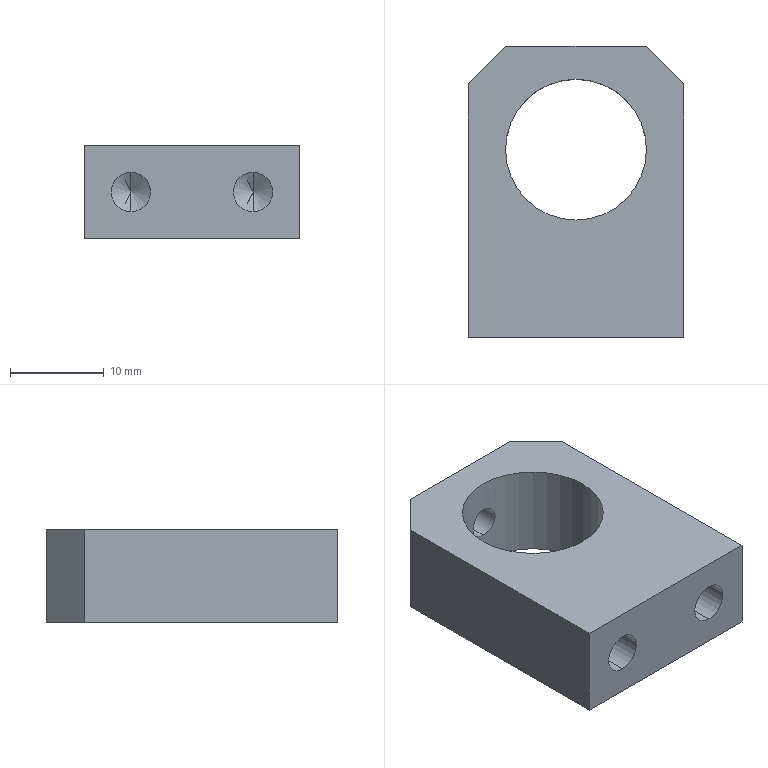Part | SolidWorks | features 3DProfileFeature 3, HoleWzd 3, ICE 2, Chamfer 1, Extrusion 1 | 1 solid | 20 faces | box 23 x 31 x 10 mm | volume 4928 mm3 | cylinder 8 | plane 8 | cone 4 | commonest cylinder face diameters 4.2 x4 3.3 x2 15 x2
STEP:
#1=CARTESIAN_POINT('',(-6.5,8.4,2.1));
#2=VERTEX_POINT('',#1);
#3=CARTESIAN_POINT('',(-6.5,8.4,-2.1));
#4=VERTEX_POINT('',#3);
#5=CARTESIAN_POINT('',(-6.5,8.4,0.));
#6=DIRECTION('',(0.,-1.,0.));
#7=DIRECTION('',(0.,0.,-1.));
#8=AXIS2_PLACEMENT_3D('',#5,#6,#7);
#9=CIRCLE('',#8,2.1);
#10=EDGE_CURVE('',#2,#4,#9,.T.);
#11=ORIENTED_EDGE('',*,*,#10,.F.);
#12=CARTESIAN_POINT('',(-6.5,0.,2.1));
#13=VERTEX_POINT('',#12);
#14=CARTESIAN_POINT('',(-6.5,0.,2.1));
#15=DIRECTION('',(0.,-1.,0.));
#16=VECTOR('',#15,1000.);
#17=LINE('',#14,#16);
#18=EDGE_CURVE('',#2,#13,#17,.T.);
#19=ORIENTED_EDGE('',*,*,#18,.T.);
#20=CARTESIAN_POINT('',(-6.5,0.,-2.1));
#21=VERTEX_POINT('',#20);
#22=CARTESIAN_POINT('',(-6.5,0.,0.));
#23=DIRECTION('',(0.,-1.,0.));
#24=DIRECTION('',(0.,0.,-1.));
#25=AXIS2_PLACEMENT_3D('',#22,#23,#24);
#26=CIRCLE('',#25,2.1);
#27=EDGE_CURVE('',#13,#21,#26,.T.);
#28=ORIENTED_EDGE('',*,*,#27,.T.);
#29=CARTESIAN_POINT('',(-6.5,0.,-2.1));
#30=DIRECTION('',(0.,-1.,0.));
#31=VECTOR('',#30,1000.);
#32=LINE('',#29,#31);
#33=EDGE_CURVE('',#4,#21,#32,.T.);
#34=ORIENTED_EDGE('',*,*,#33,.F.);
#35=EDGE_LOOP('',(#11,#19,#28,#34));
#36=FACE_OUTER_BOUND('',#35,.T.);
#37=CARTESIAN_POINT('',(-6.5,0.,0.));
#38=DIRECTION('',(0.,-1.,0.));
#39=DIRECTION('',(0.,0.,-1.));
#40=AXIS2_PLACEMENT_3D('',#37,#38,#39);
#41=CYLINDRICAL_SURFACE('',#40,2.1);
#42=ADVANCED_FACE('',(#36),#41,.F.);
#43=CARTESIAN_POINT('',(-6.5,9.662,0.));
#44=VERTEX_POINT('',#43);
#45=CARTESIAN_POINT('',(-6.5,8.4,-2.1));
#46=DIRECTION('',(0.,-0.515,-0.8572));
#47=VECTOR('',#46,1000.);
#48=LINE('',#45,#47);
#49=EDGE_CURVE('',#44,#4,#48,.T.);
#50=ORIENTED_EDGE('',*,*,#49,.F.);
#51=CARTESIAN_POINT('',(-6.5,8.4,2.1));
#52=DIRECTION('',(0.,-0.515,0.8572));
#53=VECTOR('',#52,1000.);
#54=LINE('',#51,#53);
#55=EDGE_CURVE('',#44,#2,#54,.T.);
#56=ORIENTED_EDGE('',*,*,#55,.T.);
#57=ORIENTED_EDGE('',*,*,#10,.T.);
#58=EDGE_LOOP('',(#50,#56,#57));
#59=FACE_OUTER_BOUND('',#58,.T.);
#60=CARTESIAN_POINT('',(-6.5,8.4,0.));
#61=DIRECTION('',(0.,-1.,0.));
#62=DIRECTION('',(0.,0.,-1.));
#63=AXIS2_PLACEMENT_3D('',#60,#61,#62);
#64=CONICAL_SURFACE('',#63,2.1,1.03);
#65=ADVANCED_FACE('',(#59),#64,.F.);
#66=CARTESIAN_POINT('',(6.5,8.4,2.1));
#67=VERTEX_POINT('',#66);
#68=CARTESIAN_POINT('',(6.5,8.4,-2.1));
#69=VERTEX_POINT('',#68);
#70=CARTESIAN_POINT('',(6.5,8.4,0.));
#71=DIRECTION('',(0.,-1.,0.));
#72=DIRECTION('',(0.,0.,-1.));
#73=AXIS2_PLACEMENT_3D('',#70,#71,#72);
#74=CIRCLE('',#73,2.1);
#75=EDGE_CURVE('',#67,#69,#74,.T.);
#76=ORIENTED_EDGE('',*,*,#75,.F.);
#77=CARTESIAN_POINT('',(6.5,0.,2.1));
#78=VERTEX_POINT('',#77);
#79=CARTESIAN_POINT('',(6.5,0.,2.1));
#80=DIRECTION('',(0.,-1.,0.));
#81=VECTOR('',#80,1000.);
#82=LINE('',#79,#81);
#83=EDGE_CURVE('',#67,#78,#82,.T.);
#84=ORIENTED_EDGE('',*,*,#83,.T.);
#85=CARTESIAN_POINT('',(6.5,0.,-2.1));
#86=VERTEX_POINT('',#85);
#87=CARTESIAN_POINT('',(6.5,0.,0.));
#88=DIRECTION('',(0.,-1.,0.));
#89=DIRECTION('',(0.,0.,-1.));
#90=AXIS2_PLACEMENT_3D('',#87,#88,#89);
#91=CIRCLE('',#90,2.1);
#92=EDGE_CURVE('',#78,#86,#91,.T.);
#93=ORIENTED_EDGE('',*,*,#92,.T.);
#94=CARTESIAN_POINT('',(6.5,0.,-2.1));
#95=DIRECTION('',(0.,-1.,0.));
#96=VECTOR('',#95,1000.);
#97=LINE('',#94,#96);
#98=EDGE_CURVE('',#69,#86,#97,.T.);
#99=ORIENTED_EDGE('',*,*,#98,.F.);
#100=EDGE_LOOP('',(#76,#84,#93,#99));
#101=FACE_OUTER_BOUND('',#100,.T.);
#102=CARTESIAN_POINT('',(6.5,0.,0.));
#103=DIRECTION('',(0.,-1.,0.));
#104=DIRECTION('',(0.,0.,-1.));
#105=AXIS2_PLACEMENT_3D('',#102,#103,#104);
#106=CYLINDRICAL_SURFACE('',#105,2.1);
#107=ADVANCED_FACE('',(#101),#106,.F.);
#108=CARTESIAN_POINT('',(6.5,9.662,0.));
#109=VERTEX_POINT('',#108);
#110=CARTESIAN_POINT('',(6.5,8.4,-2.1));
#111=DIRECTION('',(0.,-0.515,-0.8572));
#112=VECTOR('',#111,1000.);
#113=LINE('',#110,#112);
#114=EDGE_CURVE('',#109,#69,#113,.T.);
#115=ORIENTED_EDGE('',*,*,#114,.F.);
#116=CARTESIAN_POINT('',(6.5,8.4,2.1));
#117=DIRECTION('',(0.,-0.515,0.8572));
#118=VECTOR('',#117,1000.);
#119=LINE('',#116,#118);
#120=EDGE_CURVE('',#109,#67,#119,.T.);
#121=ORIENTED_EDGE('',*,*,#120,.T.);
#122=ORIENTED_EDGE('',*,*,#75,.T.);
#123=EDGE_LOOP('',(#115,#121,#122));
#124=FACE_OUTER_BOUND('',#123,.T.);
#125=CARTESIAN_POINT('',(6.5,8.4,0.));
#126=DIRECTION('',(0.,-1.,0.));
#127=DIRECTION('',(0.,0.,-1.));
#128=AXIS2_PLACEMENT_3D('',#125,#126,#127);
#129=CONICAL_SURFACE('',#128,2.1,1.03);
#130=ADVANCED_FACE('',(#124),#129,.F.);
#131=CARTESIAN_POINT('',(0.,27.5,1.65));
#132=VERTEX_POINT('',#131);
#133=CARTESIAN_POINT('',(0.,27.5,-1.65));
#134=VERTEX_POINT('',#133);
#135=CARTESIAN_POINT('',(0.,27.5,1.65));
#136=CARTESIAN_POINT('',(-0.1094,27.5,1.65));
#137=CARTESIAN_POINT('',(-0.2169,27.498,1.639));
#138=CARTESIAN_POINT('',(-0.4282,27.489,1.597));
#139=CARTESIAN_POINT('',(-0.5332,27.482,1.565));
#140=CARTESIAN_POINT('',(-0.7329,27.465,1.482));
#141=CARTESIAN_POINT('',(-0.8275,27.455,1.432));
#142=CARTESIAN_POINT('',(-1.007,27.433,1.312));
#143=CARTESIAN_POINT('',(-1.091,27.421,1.242));
#144=CARTESIAN_POINT('',(-1.319,27.385,1.015));
#145=CARTESIAN_POINT('',(-1.442,27.361,0.8311));
#146=CARTESIAN_POINT('',(-1.606,27.326,0.4343));
#147=CARTESIAN_POINT('',(-1.65,27.316,0.2166));
#148=CARTESIAN_POINT('',(-1.65,27.316,-0.1073));
#149=CARTESIAN_POINT('',(-1.639,27.319,-0.2171));
#150=CARTESIAN_POINT('',(-1.597,27.328,-0.4289));
#151=CARTESIAN_POINT('',(-1.566,27.335,-0.532));
#152=CARTESIAN_POINT('',(-1.441,27.361,-0.8322));
#153=CARTESIAN_POINT('',(-1.32,27.385,-1.014));
#154=CARTESIAN_POINT('',(-1.09,27.421,-1.243));
#155=CARTESIAN_POINT('',(-1.007,27.433,-1.311));
#156=CARTESIAN_POINT('',(-0.8286,27.455,-1.431));
#157=CARTESIAN_POINT('',(-0.7319,27.465,-1.483));
#158=CARTESIAN_POINT('',(-0.5325,27.482,-1.565));
#159=CARTESIAN_POINT('',(-0.4297,27.488,-1.597));
#160=CARTESIAN_POINT('',(-0.2174,27.498,-1.639));
#161=CARTESIAN_POINT('',(-0.1079,27.5,-1.65));
#162=CARTESIAN_POINT('',(0.,27.5,-1.65));
#163=B_SPLINE_CURVE_WITH_KNOTS('',3,(#135,#136,#137,#138,#139,#140,#141,#142,#143,#144,#145,#146,#147,#148,#149,#150,#151,#152,#153,#154,#155,#156,#157,#158,#159,#160,#161,#162),.UNSPECIFIED.,.F.,.F.,(4,2,2,2,2,2,2,2,2,2,2,2,2,4),(0.,0.0003234,0.0006468,0.0009702,0.001294,0.00194,0.002587,0.002911,0.003234,0.003881,0.004204,0.004528,0.004851,0.005175),.UNSPECIFIED.);
#164=EDGE_CURVE('',#132,#134,#163,.T.);
#165=ORIENTED_EDGE('',*,*,#164,.T.);
#166=CARTESIAN_POINT('',(0.,31.,-1.65));
#167=VERTEX_POINT('',#166);
#168=CARTESIAN_POINT('',(0.,31.,-1.65));
#169=DIRECTION('',(0.,1.,0.));
#170=VECTOR('',#169,1000.);
#171=LINE('',#168,#170);
#172=EDGE_CURVE('',#134,#167,#171,.T.);
#173=ORIENTED_EDGE('',*,*,#172,.T.);
#174=CARTESIAN_POINT('',(0.,31.,1.65));
#175=VERTEX_POINT('',#174);
#176=CARTESIAN_POINT('',(0.,31.,0.));
#177=DIRECTION('',(0.,1.,0.));
#178=DIRECTION('',(0.,0.,1.));
#179=AXIS2_PLACEMENT_3D('',#176,#177,#178);
#180=CIRCLE('',#179,1.65);
#181=EDGE_CURVE('',#167,#175,#180,.T.);
#182=ORIENTED_EDGE('',*,*,#181,.T.);
#183=CARTESIAN_POINT('',(0.,31.,1.65));
#184=DIRECTION('',(0.,1.,0.));
#185=VECTOR('',#184,1000.);
#186=LINE('',#183,#185);
#187=EDGE_CURVE('',#132,#175,#186,.T.);
#188=ORIENTED_EDGE('',*,*,#187,.F.);
#189=EDGE_LOOP('',(#165,#173,#182,#188));
#190=FACE_OUTER_BOUND('',#189,.T.);
#191=CARTESIAN_POINT('',(0.,31.,0.));
#192=DIRECTION('',(0.,1.,0.));
#193=DIRECTION('',(0.,0.,1.));
#194=AXIS2_PLACEMENT_3D('',#191,#192,#193);
#195=CYLINDRICAL_SURFACE('',#194,1.65);
#196=ADVANCED_FACE('',(#190),#195,.F.);
#197=CARTESIAN_POINT('',(-7.5,20.,5.));
#198=VERTEX_POINT('',#197);
#199=CARTESIAN_POINT('',(7.5,20.,5.));
#200=VERTEX_POINT('',#199);
#201=CARTESIAN_POINT('',(0.,20.,5.));
#202=DIRECTION('',(0.,0.,1.));
#203=DIRECTION('',(1.,0.,0.));
#204=AXIS2_PLACEMENT_3D('',#201,#202,#203);
#205=CIRCLE('',#204,7.5);
#206=EDGE_CURVE('',#198,#200,#205,.T.);
#207=ORIENTED_EDGE('',*,*,#206,.T.);
#208=CARTESIAN_POINT('',(7.5,20.,-5.));
#209=VERTEX_POINT('',#208);
#210=CARTESIAN_POINT('',(7.5,20.,5.));
#211=DIRECTION('',(0.,0.,-1.));
#212=VECTOR('',#211,1000.);
#213=LINE('',#210,#212);
#214=EDGE_CURVE('',#200,#209,#213,.T.);
#215=ORIENTED_EDGE('',*,*,#214,.T.);
#216=CARTESIAN_POINT('',(-7.5,20.,-5.));
#217=VERTEX_POINT('',#216);
#218=CARTESIAN_POINT('',(0.,20.,-5.));
#219=DIRECTION('',(0.,0.,1.));
#220=DIRECTION('',(1.,0.,0.));
#221=AXIS2_PLACEMENT_3D('',#218,#219,#220);
#222=CIRCLE('',#221,7.5);
#223=EDGE_CURVE('',#217,#209,#222,.T.);
#224=ORIENTED_EDGE('',*,*,#223,.F.);
#225=CARTESIAN_POINT('',(-7.5,20.,5.));
#226=DIRECTION('',(0.,0.,-1.));
#227=VECTOR('',#226,1000.);
#228=LINE('',#225,#227);
#229=EDGE_CURVE('',#198,#217,#228,.T.);
#230=ORIENTED_EDGE('',*,*,#229,.F.);
#231=EDGE_LOOP('',(#207,#215,#224,#230));
#232=FACE_OUTER_BOUND('',#231,.T.);
#233=CARTESIAN_POINT('',(0.,20.,5.));
#234=DIRECTION('',(0.,0.,-1.));
#235=DIRECTION('',(-1.,0.,0.));
#236=AXIS2_PLACEMENT_3D('',#233,#234,#235);
#237=CYLINDRICAL_SURFACE('',#236,7.5);
#238=ADVANCED_FACE('',(#232),#237,.F.);
#239=CARTESIAN_POINT('',(7.5,31.,5.));
#240=VERTEX_POINT('',#239);
#241=CARTESIAN_POINT('',(-7.5,31.,5.));
#242=VERTEX_POINT('',#241);
#243=CARTESIAN_POINT('',(-11.5,31.,5.));
#244=DIRECTION('',(-1.,0.,0.));
#245=VECTOR('',#244,1000.);
#246=LINE('',#243,#245);
#247=EDGE_CURVE('',#240,#242,#246,.T.);
#248=ORIENTED_EDGE('',*,*,#247,.T.);
#249=CARTESIAN_POINT('',(-11.5,27.,5.));
#250=VERTEX_POINT('',#249);
#251=CARTESIAN_POINT('',(-11.5,27.,5.));
#252=DIRECTION('',(-0.7071,-0.7071,0.));
#253=VECTOR('',#252,1000.);
#254=LINE('',#251,#253);
#255=EDGE_CURVE('',#242,#250,#254,.T.);
#256=ORIENTED_EDGE('',*,*,#255,.T.);
#257=CARTESIAN_POINT('',(-11.5,0.,5.));
#258=VERTEX_POINT('',#257);
#259=CARTESIAN_POINT('',(-11.5,0.,5.));
#260=DIRECTION('',(0.,-1.,0.));
#261=VECTOR('',#260,1000.);
#262=LINE('',#259,#261);
#263=EDGE_CURVE('',#250,#258,#262,.T.);
#264=ORIENTED_EDGE('',*,*,#263,.T.);
#265=CARTESIAN_POINT('',(11.5,0.,5.));
#266=VERTEX_POINT('',#265);
#267=CARTESIAN_POINT('',(-11.5,0.,5.));
#268=DIRECTION('',(1.,0.,0.));
#269=VECTOR('',#268,1000.);
#270=LINE('',#267,#269);
#271=EDGE_CURVE('',#258,#266,#270,.T.);
#272=ORIENTED_EDGE('',*,*,#271,.T.);
#273=CARTESIAN_POINT('',(11.5,27.,5.));
#274=VERTEX_POINT('',#273);
#275=CARTESIAN_POINT('',(11.5,31.,5.));
#276=DIRECTION('',(0.,1.,0.));
#277=VECTOR('',#276,1000.);
#278=LINE('',#275,#277);
#279=EDGE_CURVE('',#266,#274,#278,.T.);
#280=ORIENTED_EDGE('',*,*,#279,.T.);
#281=CARTESIAN_POINT('',(7.5,31.,5.));
#282=DIRECTION('',(-0.7071,0.7071,0.));
#283=VECTOR('',#282,1000.);
#284=LINE('',#281,#283);
#285=EDGE_CURVE('',#274,#240,#284,.T.);
#286=ORIENTED_EDGE('',*,*,#285,.T.);
#287=EDGE_LOOP('',(#248,#256,#264,#272,#280,#286));
#288=FACE_OUTER_BOUND('',#287,.T.);
#289=ORIENTED_EDGE('',*,*,#206,.F.);
#290=CARTESIAN_POINT('',(0.,20.,5.));
#291=DIRECTION('',(0.,0.,1.));
#292=DIRECTION('',(1.,0.,0.));
#293=AXIS2_PLACEMENT_3D('',#290,#291,#292);
#294=CIRCLE('',#293,7.5);
#295=EDGE_CURVE('',#200,#198,#294,.T.);
#296=ORIENTED_EDGE('',*,*,#295,.F.);
#297=EDGE_LOOP('',(#289,#296));
#298=FACE_BOUND('',#297,.T.);
#299=CARTESIAN_POINT('',(0.,0.,5.));
#300=DIRECTION('',(0.,0.,-1.));
#301=DIRECTION('',(-1.,0.,0.));
#302=AXIS2_PLACEMENT_3D('',#299,#300,#301);
#303=PLANE('',#302);
#304=ADVANCED_FACE('',(#288,#298),#303,.F.);
#305=CARTESIAN_POINT('',(-11.5,27.,-5.));
#306=VERTEX_POINT('',#305);
#307=CARTESIAN_POINT('',(-11.5,0.,-5.));
#308=VERTEX_POINT('',#307);
#309=CARTESIAN_POINT('',(-11.5,0.,-5.));
#310=DIRECTION('',(0.,-1.,0.));
#311=VECTOR('',#310,1000.);
#312=LINE('',#309,#311);
#313=EDGE_CURVE('',#306,#308,#312,.T.);
#314=ORIENTED_EDGE('',*,*,#313,.F.);
#315=CARTESIAN_POINT('',(-7.5,31.,-5.));
#316=VERTEX_POINT('',#315);
#317=CARTESIAN_POINT('',(-19.25,19.25,-5.));
#318=DIRECTION('',(0.7071,0.7071,0.));
#319=VECTOR('',#318,1000.);
#320=LINE('',#317,#319);
#321=EDGE_CURVE('',#306,#316,#320,.T.);
#322=ORIENTED_EDGE('',*,*,#321,.T.);
#323=CARTESIAN_POINT('',(7.5,31.,-5.));
#324=VERTEX_POINT('',#323);
#325=CARTESIAN_POINT('',(-11.5,31.,-5.));
#326=DIRECTION('',(-1.,0.,0.));
#327=VECTOR('',#326,1000.);
#328=LINE('',#325,#327);
#329=EDGE_CURVE('',#324,#316,#328,.T.);
#330=ORIENTED_EDGE('',*,*,#329,.F.);
#331=CARTESIAN_POINT('',(11.5,27.,-5.));
#332=VERTEX_POINT('',#331);
#333=CARTESIAN_POINT('',(19.25,19.25,-5.));
#334=DIRECTION('',(0.7071,-0.7071,0.));
#335=VECTOR('',#334,1000.);
#336=LINE('',#333,#335);
#337=EDGE_CURVE('',#324,#332,#336,.T.);
#338=ORIENTED_EDGE('',*,*,#337,.T.);
#339=CARTESIAN_POINT('',(11.5,0.,-5.));
#340=VERTEX_POINT('',#339);
#341=CARTESIAN_POINT('',(11.5,31.,-5.));
#342=DIRECTION('',(0.,1.,0.));
#343=VECTOR('',#342,1000.);
#344=LINE('',#341,#343);
#345=EDGE_CURVE('',#340,#332,#344,.T.);
#346=ORIENTED_EDGE('',*,*,#345,.F.);
#347=CARTESIAN_POINT('',(-11.5,0.,-5.));
#348=DIRECTION('',(1.,0.,0.));
#349=VECTOR('',#348,1000.);
#350=LINE('',#347,#349);
#351=EDGE_CURVE('',#308,#340,#350,.T.);
#352=ORIENTED_EDGE('',*,*,#351,.F.);
#353=EDGE_LOOP('',(#314,#322,#330,#338,#346,#352));
#354=FACE_OUTER_BOUND('',#353,.T.);
#355=ORIENTED_EDGE('',*,*,#223,.T.);
#356=CARTESIAN_POINT('',(0.,20.,-5.));
#357=DIRECTION('',(0.,0.,1.));
#358=DIRECTION('',(1.,0.,0.));
#359=AXIS2_PLACEMENT_3D('',#356,#357,#358);
#360=CIRCLE('',#359,7.5);
#361=EDGE_CURVE('',#209,#217,#360,.T.);
#362=ORIENTED_EDGE('',*,*,#361,.T.);
#363=EDGE_LOOP('',(#355,#362));
#364=FACE_BOUND('',#363,.T.);
#365=CARTESIAN_POINT('',(0.,0.,-5.));
#366=DIRECTION('',(0.,0.,-1.));
#367=DIRECTION('',(-1.,0.,0.));
#368=AXIS2_PLACEMENT_3D('',#365,#366,#367);
#369=PLANE('',#368);
#370=ADVANCED_FACE('',(#354,#364),#369,.T.);
#371=CARTESIAN_POINT('',(0.,31.,0.));
#372=DIRECTION('',(0.,1.,0.));
#373=DIRECTION('',(0.,0.,1.));
#374=AXIS2_PLACEMENT_3D('',#371,#372,#373);
#375=CIRCLE('',#374,1.65);
#376=EDGE_CURVE('',#175,#167,#375,.T.);
#377=ORIENTED_EDGE('',*,*,#376,.F.);
#378=ORIENTED_EDGE('',*,*,#181,.F.);
#379=EDGE_LOOP('',(#377,#378));
#380=FACE_BOUND('',#379,.T.);
#381=ORIENTED_EDGE('',*,*,#329,.T.);
#382=CARTESIAN_POINT('',(-7.5,31.,5.));
#383=DIRECTION('',(0.,0.,1.));
#384=VECTOR('',#383,1000.);
#385=LINE('',#382,#384);
#386=EDGE_CURVE('',#316,#242,#385,.T.);
#387=ORIENTED_EDGE('',*,*,#386,.T.);
#388=ORIENTED_EDGE('',*,*,#247,.F.);
#389=CARTESIAN_POINT('',(7.5,31.,5.));
#390=DIRECTION('',(0.,0.,-1.));
#391=VECTOR('',#390,1000.);
#392=LINE('',#389,#391);
#393=EDGE_CURVE('',#240,#324,#392,.T.);
#394=ORIENTED_EDGE('',*,*,#393,.T.);
#395=EDGE_LOOP('',(#381,#387,#388,#394));
#396=FACE_OUTER_BOUND('',#395,.T.);
#397=CARTESIAN_POINT('',(-11.5,31.,5.));
#398=DIRECTION('',(0.,-1.,0.));
#399=DIRECTION('',(0.,0.,-1.));
#400=AXIS2_PLACEMENT_3D('',#397,#398,#399);
#401=PLANE('',#400);
#402=ADVANCED_FACE('',(#380,#396),#401,.F.);
#403=ORIENTED_EDGE('',*,*,#263,.F.);
#404=CARTESIAN_POINT('',(-11.5,27.,5.));
#405=DIRECTION('',(0.,0.,-1.));
#406=VECTOR('',#405,1000.);
#407=LINE('',#404,#406);
#408=EDGE_CURVE('',#250,#306,#407,.T.);
#409=ORIENTED_EDGE('',*,*,#408,.T.);
#410=ORIENTED_EDGE('',*,*,#313,.T.);
#411=CARTESIAN_POINT('',(-11.5,0.,5.));
#412=DIRECTION('',(0.,0.,-1.));
#413=VECTOR('',#412,1000.);
#414=LINE('',#411,#413);
#415=EDGE_CURVE('',#258,#308,#414,.T.);
#416=ORIENTED_EDGE('',*,*,#415,.F.);
#417=EDGE_LOOP('',(#403,#409,#410,#416));
#418=FACE_OUTER_BOUND('',#417,.T.);
#419=CARTESIAN_POINT('',(-11.5,0.,5.));
#420=DIRECTION('',(1.,0.,0.));
#421=DIRECTION('',(0.,0.,-1.));
#422=AXIS2_PLACEMENT_3D('',#419,#420,#421);
#423=PLANE('',#422);
#424=ADVANCED_FACE('',(#418),#423,.F.);
#425=CARTESIAN_POINT('',(-6.5,0.,0.));
#426=DIRECTION('',(0.,-1.,0.));
#427=DIRECTION('',(0.,0.,-1.));
#428=AXIS2_PLACEMENT_3D('',#425,#426,#427);
#429=CIRCLE('',#428,2.1);
#430=EDGE_CURVE('',#21,#13,#429,.T.);
#431=ORIENTED_EDGE('',*,*,#430,.F.);
#432=ORIENTED_EDGE('',*,*,#27,.F.);
#433=EDGE_LOOP('',(#431,#432));
#434=FACE_BOUND('',#433,.T.);
#435=CARTESIAN_POINT('',(6.5,0.,0.));
#436=DIRECTION('',(0.,-1.,0.));
#437=DIRECTION('',(0.,0.,-1.));
#438=AXIS2_PLACEMENT_3D('',#435,#436,#437);
#439=CIRCLE('',#438,2.1);
#440=EDGE_CURVE('',#86,#78,#439,.T.);
#441=ORIENTED_EDGE('',*,*,#440,.F.);
#442=ORIENTED_EDGE('',*,*,#92,.F.);
#443=EDGE_LOOP('',(#441,#442));
#444=FACE_BOUND('',#443,.T.);
#445=ORIENTED_EDGE('',*,*,#351,.T.);
#446=CARTESIAN_POINT('',(11.5,0.,5.));
#447=DIRECTION('',(0.,0.,-1.));
#448=VECTOR('',#447,1000.);
#449=LINE('',#446,#448);
#450=EDGE_CURVE('',#266,#340,#449,.T.);
#451=ORIENTED_EDGE('',*,*,#450,.F.);
#452=ORIENTED_EDGE('',*,*,#271,.F.);
#453=ORIENTED_EDGE('',*,*,#415,.T.);
#454=EDGE_LOOP('',(#445,#451,#452,#453));
#455=FACE_OUTER_BOUND('',#454,.T.);
#456=CARTESIAN_POINT('',(-11.5,0.,5.));
#457=DIRECTION('',(0.,1.,0.));
#458=DIRECTION('',(0.,0.,1.));
#459=AXIS2_PLACEMENT_3D('',#456,#457,#458);
#460=PLANE('',#459);
#461=ADVANCED_FACE('',(#434,#444,#455),#460,.F.);
#462=ORIENTED_EDGE('',*,*,#345,.T.);
#463=CARTESIAN_POINT('',(11.5,27.,5.));
#464=DIRECTION('',(0.,0.,1.));
#465=VECTOR('',#464,1000.);
#466=LINE('',#463,#465);
#467=EDGE_CURVE('',#332,#274,#466,.T.);
#468=ORIENTED_EDGE('',*,*,#467,.T.);
#469=ORIENTED_EDGE('',*,*,#279,.F.);
#470=ORIENTED_EDGE('',*,*,#450,.T.);
#471=EDGE_LOOP('',(#462,#468,#469,#470));
#472=FACE_OUTER_BOUND('',#471,.T.);
#473=CARTESIAN_POINT('',(11.5,31.,5.));
#474=DIRECTION('',(-1.,0.,0.));
#475=DIRECTION('',(0.,0.,1.));
#476=AXIS2_PLACEMENT_3D('',#473,#474,#475);
#477=PLANE('',#476);
#478=ADVANCED_FACE('',(#472),#477,.F.);
#479=ORIENTED_EDGE('',*,*,#214,.F.);
#480=ORIENTED_EDGE('',*,*,#295,.T.);
#481=ORIENTED_EDGE('',*,*,#229,.T.);
#482=ORIENTED_EDGE('',*,*,#361,.F.);
#483=EDGE_LOOP('',(#479,#480,#481,#482));
#484=FACE_OUTER_BOUND('',#483,.T.);
#485=ORIENTED_EDGE('',*,*,#164,.F.);
#486=CARTESIAN_POINT('',(0.,27.5,-1.65));
#487=CARTESIAN_POINT('',(0.2157,27.5,-1.65));
#488=CARTESIAN_POINT('',(0.4334,27.49,-1.607));
#489=CARTESIAN_POINT('',(0.7314,27.465,-1.483));
#490=CARTESIAN_POINT('',(0.8278,27.455,-1.431));
#491=CARTESIAN_POINT('',(1.007,27.433,-1.311));
#492=CARTESIAN_POINT('',(1.09,27.421,-1.243));
#493=CARTESIAN_POINT('',(1.242,27.397,-1.091));
#494=CARTESIAN_POINT('',(1.312,27.385,-1.007));
#495=CARTESIAN_POINT('',(1.431,27.362,-0.8283));
#496=CARTESIAN_POINT('',(1.482,27.352,-0.7337));
#497=CARTESIAN_POINT('',(1.607,27.326,-0.4332));
#498=CARTESIAN_POINT('',(1.65,27.316,-0.2185));
#499=CARTESIAN_POINT('',(1.65,27.316,0.1082));
#500=CARTESIAN_POINT('',(1.639,27.319,0.2155));
#501=CARTESIAN_POINT('',(1.597,27.328,0.4271));
#502=CARTESIAN_POINT('',(1.565,27.335,0.5324));
#503=CARTESIAN_POINT('',(1.442,27.361,0.8312));
#504=CARTESIAN_POINT('',(1.319,27.385,1.014));
#505=CARTESIAN_POINT('',(1.016,27.432,1.318));
#506=CARTESIAN_POINT('',(0.8326,27.456,1.441));
#507=CARTESIAN_POINT('',(0.5349,27.482,1.565));
#508=CARTESIAN_POINT('',(0.43,27.488,1.597));
#509=CARTESIAN_POINT('',(0.2172,27.498,1.639));
#510=CARTESIAN_POINT('',(0.1094,27.5,1.65));
#511=CARTESIAN_POINT('',(0.,27.5,1.65));
#512=B_SPLINE_CURVE_WITH_KNOTS('',3,(#486,#487,#488,#489,#490,#491,#492,#493,#494,#495,#496,#497,#498,#499,#500,#501,#502,#503,#504,#505,#506,#507,#508,#509,#510,#511),.UNSPECIFIED.,.F.,.F.,(4,2,2,2,2,2,2,2,2,2,2,2,4),(0.005175,0.005821,0.006144,0.006468,0.006791,0.007114,0.007761,0.008084,0.008408,0.009054,0.009701,0.01002,0.01035),.UNSPECIFIED.);
#513=EDGE_CURVE('',#134,#132,#512,.T.);
#514=ORIENTED_EDGE('',*,*,#513,.F.);
#515=EDGE_LOOP('',(#485,#514));
#516=FACE_BOUND('',#515,.T.);
#517=CARTESIAN_POINT('',(0.,20.,5.));
#518=DIRECTION('',(0.,0.,-1.));
#519=DIRECTION('',(-1.,0.,0.));
#520=AXIS2_PLACEMENT_3D('',#517,#518,#519);
#521=CYLINDRICAL_SURFACE('',#520,7.5);
#522=ADVANCED_FACE('',(#484,#516),#521,.F.);
#523=ORIENTED_EDGE('',*,*,#255,.F.);
#524=ORIENTED_EDGE('',*,*,#386,.F.);
#525=ORIENTED_EDGE('',*,*,#321,.F.);
#526=ORIENTED_EDGE('',*,*,#408,.F.);
#527=EDGE_LOOP('',(#523,#524,#525,#526));
#528=FACE_OUTER_BOUND('',#527,.T.);
#529=CARTESIAN_POINT('',(-11.5,27.,5.));
#530=DIRECTION('',(0.7071,-0.7071,0.));
#531=DIRECTION('',(0.,0.,-1.));
#532=AXIS2_PLACEMENT_3D('',#529,#530,#531);
#533=PLANE('',#532);
#534=ADVANCED_FACE('',(#528),#533,.F.);
#535=ORIENTED_EDGE('',*,*,#285,.F.);
#536=ORIENTED_EDGE('',*,*,#467,.F.);
#537=ORIENTED_EDGE('',*,*,#337,.F.);
#538=ORIENTED_EDGE('',*,*,#393,.F.);
#539=EDGE_LOOP('',(#535,#536,#537,#538));
#540=FACE_OUTER_BOUND('',#539,.T.);
#541=CARTESIAN_POINT('',(7.5,31.,5.));
#542=DIRECTION('',(-0.7071,-0.7071,0.));
#543=DIRECTION('',(0.,0.,-1.));
#544=AXIS2_PLACEMENT_3D('',#541,#542,#543);
#545=PLANE('',#544);
#546=ADVANCED_FACE('',(#540),#545,.F.);
#547=ORIENTED_EDGE('',*,*,#172,.F.);
#548=ORIENTED_EDGE('',*,*,#513,.T.);
#549=ORIENTED_EDGE('',*,*,#187,.T.);
#550=ORIENTED_EDGE('',*,*,#376,.T.);
#551=EDGE_LOOP('',(#547,#548,#549,#550));
#552=FACE_OUTER_BOUND('',#551,.T.);
#553=CARTESIAN_POINT('',(0.,31.,0.));
#554=DIRECTION('',(0.,1.,0.));
#555=DIRECTION('',(0.,0.,1.));
#556=AXIS2_PLACEMENT_3D('',#553,#554,#555);
#557=CYLINDRICAL_SURFACE('',#556,1.65);
#558=ADVANCED_FACE('',(#552),#557,.F.);
#559=ORIENTED_EDGE('',*,*,#120,.F.);
#560=ORIENTED_EDGE('',*,*,#114,.T.);
#561=CARTESIAN_POINT('',(6.5,8.4,0.));
#562=DIRECTION('',(0.,-1.,0.));
#563=DIRECTION('',(0.,0.,-1.));
#564=AXIS2_PLACEMENT_3D('',#561,#562,#563);
#565=CIRCLE('',#564,2.1);
#566=EDGE_CURVE('',#69,#67,#565,.T.);
#567=ORIENTED_EDGE('',*,*,#566,.T.);
#568=EDGE_LOOP('',(#559,#560,#567));
#569=FACE_OUTER_BOUND('',#568,.T.);
#570=CARTESIAN_POINT('',(6.5,8.4,0.));
#571=DIRECTION('',(0.,-1.,0.));
#572=DIRECTION('',(0.,0.,-1.));
#573=AXIS2_PLACEMENT_3D('',#570,#571,#572);
#574=CONICAL_SURFACE('',#573,2.1,1.03);
#575=ADVANCED_FACE('',(#569),#574,.F.);
#576=ORIENTED_EDGE('',*,*,#83,.F.);
#577=ORIENTED_EDGE('',*,*,#566,.F.);
#578=ORIENTED_EDGE('',*,*,#98,.T.);
#579=ORIENTED_EDGE('',*,*,#440,.T.);
#580=EDGE_LOOP('',(#576,#577,#578,#579));
#581=FACE_OUTER_BOUND('',#580,.T.);
#582=CARTESIAN_POINT('',(6.5,0.,0.));
#583=DIRECTION('',(0.,-1.,0.));
#584=DIRECTION('',(0.,0.,-1.));
#585=AXIS2_PLACEMENT_3D('',#582,#583,#584);
#586=CYLINDRICAL_SURFACE('',#585,2.1);
#587=ADVANCED_FACE('',(#581),#586,.F.);
#588=ORIENTED_EDGE('',*,*,#55,.F.);
#589=ORIENTED_EDGE('',*,*,#49,.T.);
#590=CARTESIAN_POINT('',(-6.5,8.4,0.));
#591=DIRECTION('',(0.,-1.,0.));
#592=DIRECTION('',(0.,0.,-1.));
#593=AXIS2_PLACEMENT_3D('',#590,#591,#592);
#594=CIRCLE('',#593,2.1);
#595=EDGE_CURVE('',#4,#2,#594,.T.);
#596=ORIENTED_EDGE('',*,*,#595,.T.);
#597=EDGE_LOOP('',(#588,#589,#596));
#598=FACE_OUTER_BOUND('',#597,.T.);
#599=CARTESIAN_POINT('',(-6.5,8.4,0.));
#600=DIRECTION('',(0.,-1.,0.));
#601=DIRECTION('',(0.,0.,-1.));
#602=AXIS2_PLACEMENT_3D('',#599,#600,#601);
#603=CONICAL_SURFACE('',#602,2.1,1.03);
#604=ADVANCED_FACE('',(#598),#603,.F.);
#605=ORIENTED_EDGE('',*,*,#18,.F.);
#606=ORIENTED_EDGE('',*,*,#595,.F.);
#607=ORIENTED_EDGE('',*,*,#33,.T.);
#608=ORIENTED_EDGE('',*,*,#430,.T.);
#609=EDGE_LOOP('',(#605,#606,#607,#608));
#610=FACE_OUTER_BOUND('',#609,.T.);
#611=CARTESIAN_POINT('',(-6.5,0.,0.));
#612=DIRECTION('',(0.,-1.,0.));
#613=DIRECTION('',(0.,0.,-1.));
#614=AXIS2_PLACEMENT_3D('',#611,#612,#613);
#615=CYLINDRICAL_SURFACE('',#614,2.1);
#616=ADVANCED_FACE('',(#610),#615,.F.);
#617=CLOSED_SHELL('',(#42,#65,#107,#130,#196,#238,#304,#370,#402,#424,#461,#478,#522,#534,#546,#558,#575,#587,#604,#616));
#618=MANIFOLD_SOLID_BREP('',#617);
#619=CARTESIAN_POINT('',(0.,0.,0.));
#620=DIRECTION('',(0.,0.,1.));
#621=DIRECTION('',(1.,0.,0.));
#622=AXIS2_PLACEMENT_3D('',#619,#620,#621);
#623=(LENGTH_UNIT()NAMED_UNIT(*)SI_UNIT(.MILLI.,.METRE.));
#624=UNCERTAINTY_MEASURE_WITH_UNIT(LENGTH_MEASURE(0.00001),#623,'','');
#625=(NAMED_UNIT(*)PLANE_ANGLE_UNIT()SI_UNIT($,.RADIAN.));
#626=(NAMED_UNIT(*)SI_UNIT($,.STERADIAN.)SOLID_ANGLE_UNIT());
#627=(GEOMETRIC_REPRESENTATION_CONTEXT(3)GLOBAL_UNCERTAINTY_ASSIGNED_CONTEXT((#624))GLOBAL_UNIT_ASSIGNED_CONTEXT((#623,#625,#626))REPRESENTATION_CONTEXT('',''));
#628=ADVANCED_BREP_SHAPE_REPRESENTATION('',(#618,#622),#627);